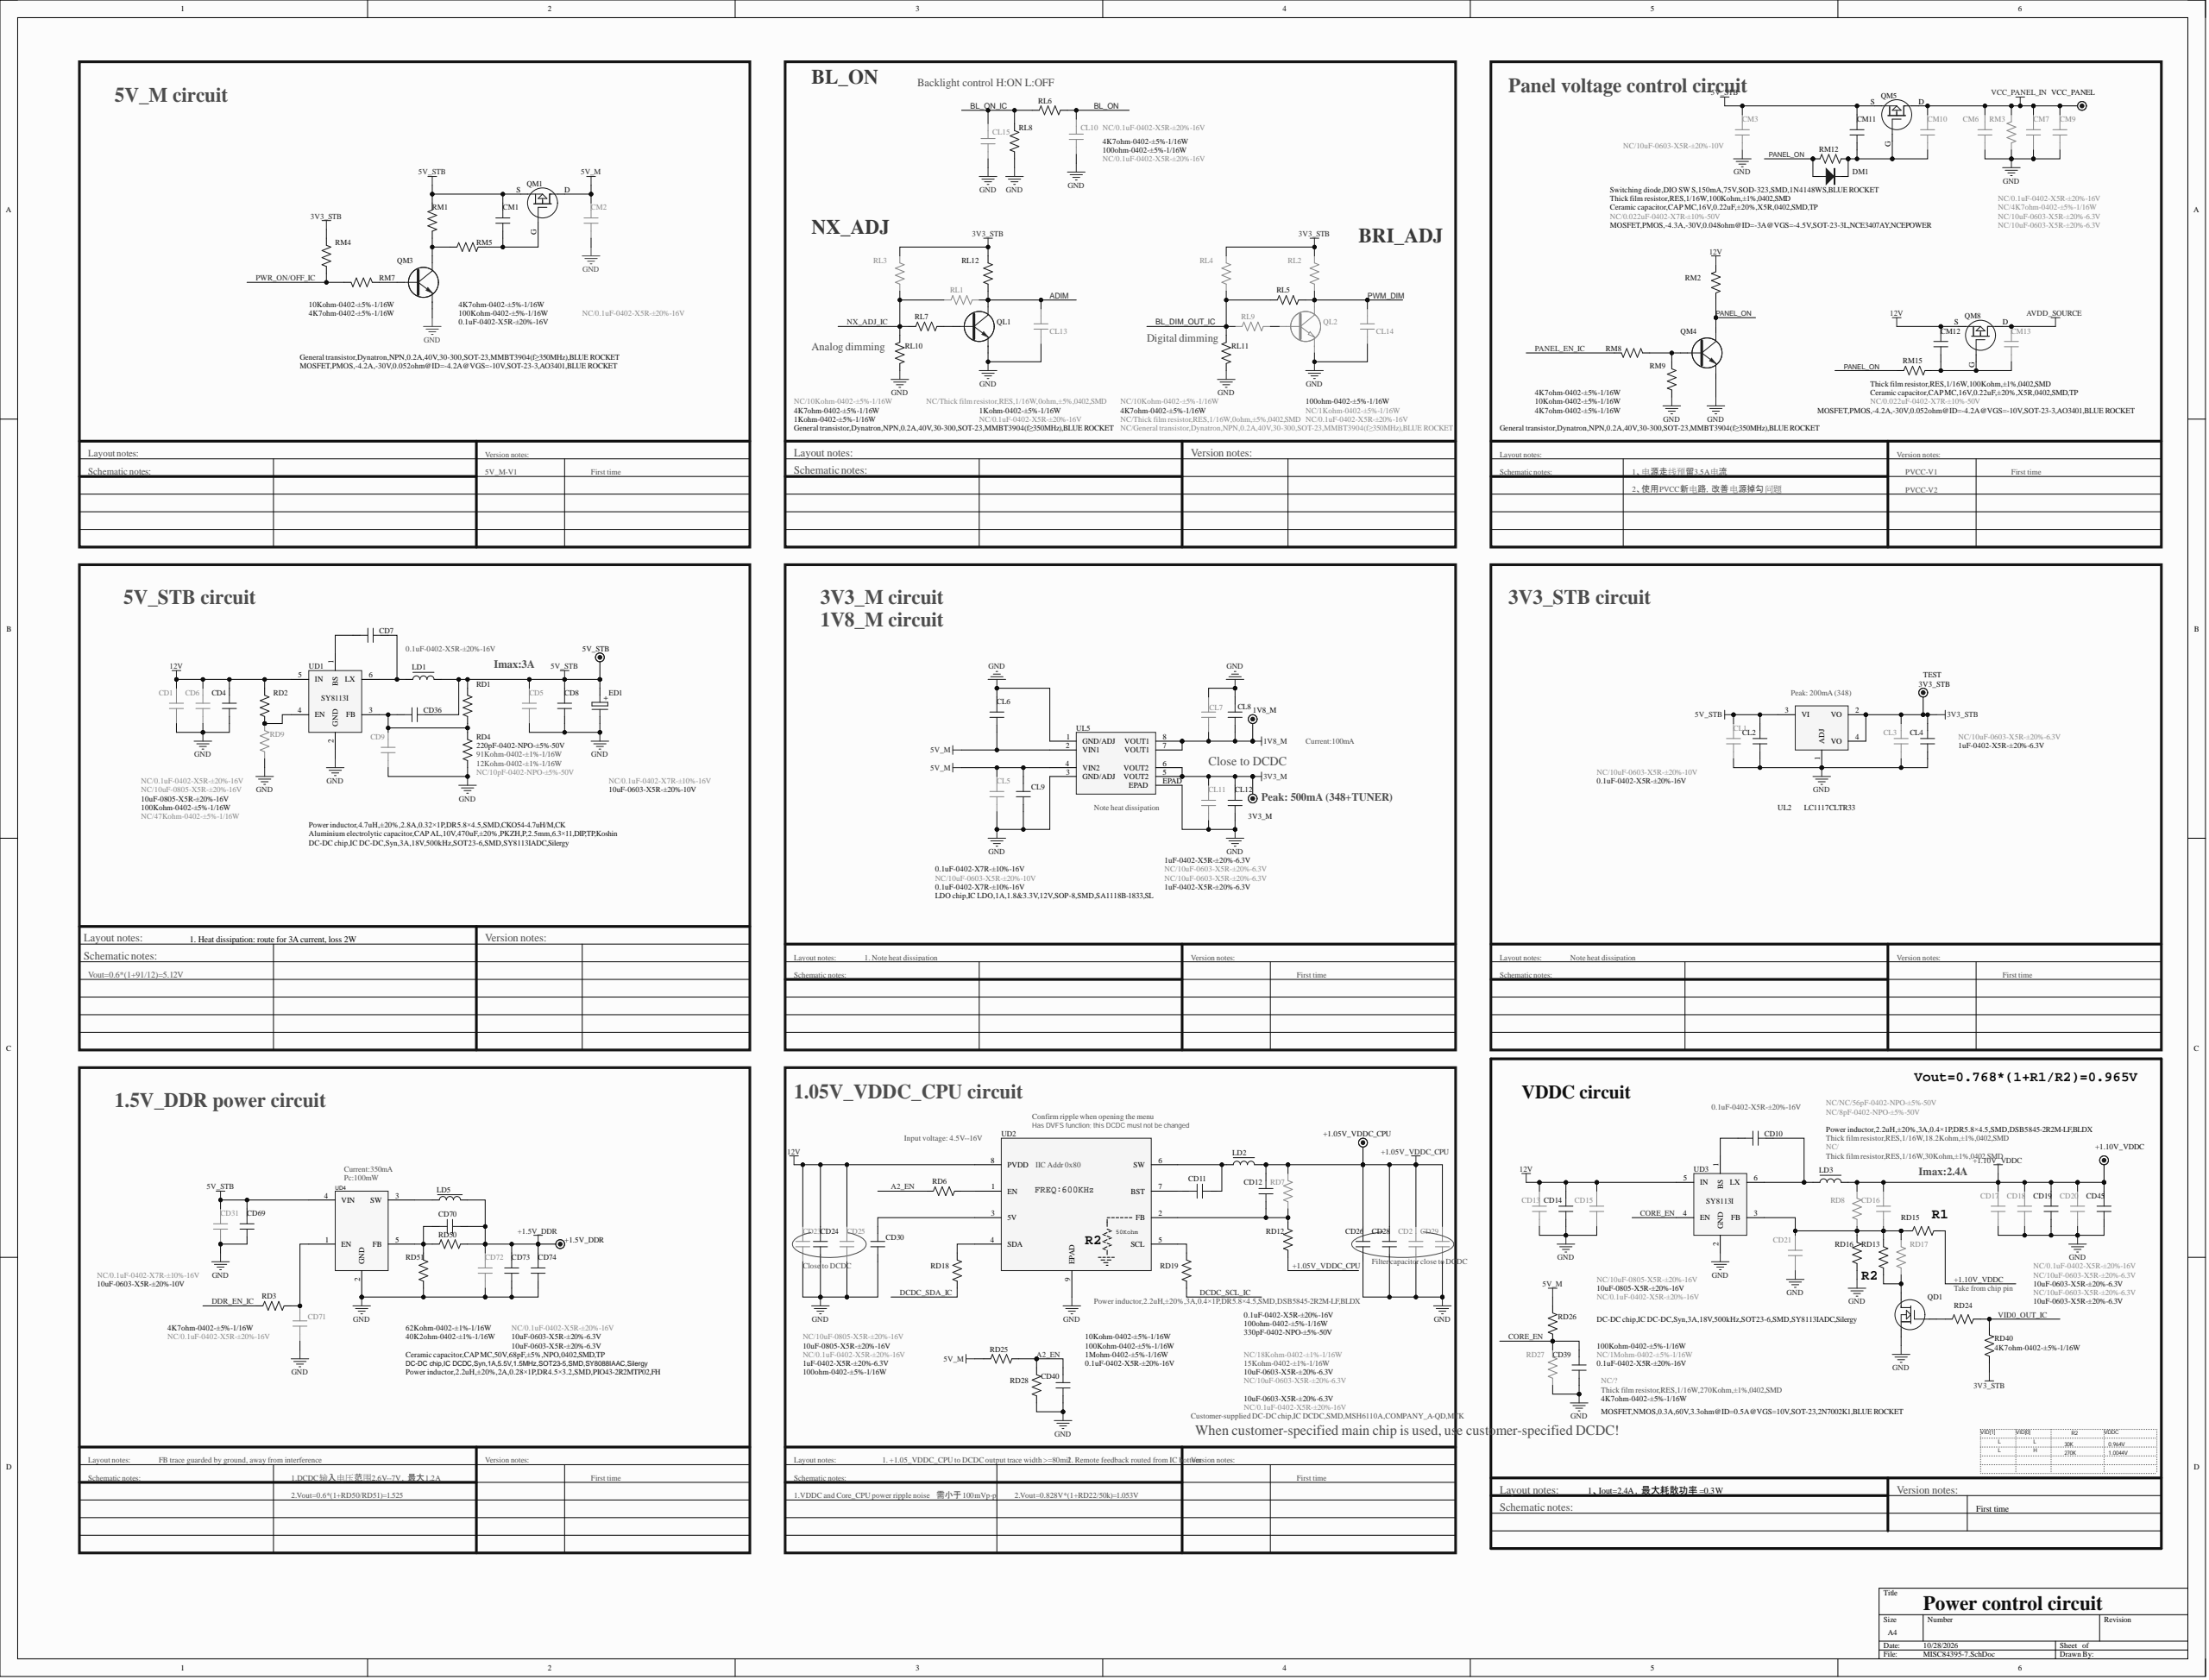Circuit board | Altium Designer | 951 parts | 509 nets | one sheet of the schematic
Parts on this sheet (reference | value | footprint):
1V8_M | TEST | TP
3V3_STB | TEST | TP
5V_STB | TEST | TP
+1.5V_DDR | TEST | TP
+1.05V_VDDC_CPU | TEST | TP
+1.10V_VDDC | TEST | TP
CD1 | NC/0.1uF-0402-X5R-±20%-16V | C0402
CD2 | NC/10uF-0603-X5R-±20%-6.3V | C0603
CD4 | 10uF-0805-X5R-±20%-16V | C0805
CD5 | NC/0.1uF-0402-X7R-±10%-16V | C0402
CD6 | NC/10uF-0805-X5R-±20%-16V | C0805
CD7 | 0.1uF-0402-X5R-±20%-16V | C0402
CD8 | 10uF-0603-X5R-±20%-10V | C0603
CD9 | NC/10pF-0402-NPO-±5%-50V | C0402
CD10 | 0.1uF-0402-X5R-±20%-16V | C0402
CD11 | 0.1uF-0402-X5R-±20%-16V | C0402
CD12 | 330pF-0402-NPO-±5%-50V | C0402
CD13 | NC/10uF-0805-X5R-±20%-16V | C0805
CD14 | 10uF-0805-X5R-±20%-16V | C0805
CD15 | NC/0.1uF-0402-X5R-±20%-16V | C0402
CD16 | NC/NC/56pF-0402-NPO-±5%-50V | C0402
CD17 | NC/0.1uF-0402-X5R-±20%-16V | C0402
CD18 | NC/10uF-0603-X5R-±20%-6.3V | C0603
CD19 | 10uF-0603-X5R-±20%-6.3V | C0603
CD20 | NC/10uF-0603-X5R-±20%-6.3V | C0603
CD21 | NC/8pF-0402-NPO-±5%-50V | C0402
CD23 | NC/10uF-0805-X5R-±20%-16V | C0805
CD24 | 10uF-0805-X5R-±20%-16V | C0805
CD25 | NC/0.1uF-0402-X5R-±20%-16V | C0402
CD26 | 10uF-0603-X5R-±20%-6.3V | C0603
CD28 | 10uF-0603-X5R-±20%-6.3V | C0603
CD29 | NC/0.1uF-0402-X5R-±20%-16V | C0402
CD30 | 1uF-0402-X5R-±20%-6.3V | C0402
CD31 | NC/0.1uF-0402-X7R-±10%-16V | C0402
CD36 | 220pF-0402-NPO-±5%-50V | C0402
CD39 | 0.1uF-0402-X5R-±20%-16V | C0402
CD40 | 0.1uF-0402-X5R-±20%-16V | C0402
CD45 | 10uF-0603-X5R-±20%-6.3V | C0603
CD69 | 10uF-0603-X5R-±20%-10V | C0603
CD70 | Ceramic capacitor,CAP MC,50V,68pF,±5%,NPO,0402,SMD,TP | C0402
CD71 | NC/0.1uF-0402-X5R-±20%-16V | C0402
CD72 | NC/0.1uF-0402-X5R-±20%-16V | C0402
CD73 | 10uF-0603-X5R-±20%-6.3V | C0603
CD74 | 10uF-0603-X5R-±20%-6.3V | C0603
CL1 | NC/10uF-0603-X5R-±20%-10V | C0603
CL2 | 0.1uF-0402-X5R-±20%-16V | C0402
CL3 | NC/10uF-0603-X5R-±20%-6.3V | C0603
CL4 | 1uF-0402-X5R-±20%-6.3V | C0402
CL5 | NC/10uF-0603-X5R-±20%-10V | C0603
CL6 | 0.1uF-0402-X7R-±10%-16V | C0402
CL7 | NC/10uF-0603-X5R-±20%-6.3V | C0603
CL8 | 1uF-0402-X5R-±20%-6.3V | C0402
CL9 | 0.1uF-0402-X7R-±10%-16V | C0402
CL10 | NC/0.1uF-0402-X5R-±20%-16V | C0402
CL11 | NC/10uF-0603-X5R-±20%-6.3V | C0603
CL12 | 1uF-0402-X5R-±20%-6.3V | C0402
CL13 | NC/0.1uF-0402-X5R-±20%-16V | C0402
CL14 | NC/0.1uF-0402-X5R-±20%-16V | C0402
CL15 | NC/0.1uF-0402-X5R-±20%-16V | C0402
CM1 | 0.1uF-0402-X5R-±20%-16V | C0402
CM2 | NC/0.1uF-0402-X5R-±20%-16V | C0402
CM3 | NC/10uF-0603-X5R-±20%-10V | C0603
CM6 | NC/0.1uF-0402-X5R-±20%-16V | C0402
CM7 | NC/10uF-0603-X5R-±20%-6.3V | C0603
CM9 | NC/10uF-0603-X5R-±20%-6.3V | C0603
CM10 | NC/0.022uF-0402-X7R-±10%-50V | C0402
CM11 | Ceramic capacitor,CAP MC,16V,0.22uF,±20%,X5R,0402,SMD,TP | C0402
CM12 | Ceramic capacitor,CAP MC,16V,0.22uF,±20%,X5R,0402,SMD,TP | C0402
CM13 | NC/0.022uF-0402-X7R-±10%-50V | C0402
DM1 | Switching diode,DIO SW S,150mA,75V,SOD-323,SMD,1N4148WS,BLUE ROCKET | DIODE-S-12
ED1 | Aluminium electrolytic capacitor,CAP AL,10V,470uF,±20%,PKZH,P,2.5mm,6.3×11,DIP,TP,Koshin | EC(6.3*11)-V-2.5
LD1 | Power inductor,4.7uH,±20%,2.8A,0.32×1P,DR5.8×4.5,SMD,CKO54-4.7uH/M,CK | L(6.0*4.5)-S
LD2 | Power inductor,2.2uH,±20%,3A,0.4×1P,DR5.8×4.5,SMD,DSB5845-2R2M-LF,BLDX | L(5.8*4.5)-S
LD3 | Power inductor,2.2uH,±20%,3A,0.4×1P,DR5.8×4.5,SMD,DSB5845-2R2M-LF,BLDX | L(5.8*4.5)-S
LD5 | Power inductor,2.2uH,±20%,2A,0.28×1P,DR4.5×3.2,SMD,PIO43-2R2MTP02,FH | L(4.5*3.5)-S
QD1 | MOSFET,NMOS,0.3A,60V,3.3ohm@ID=0.5A@VGS=10V,SOT-23,2N7002K1,BLUE ROCKET | SOT-23-7
QL1 | General transistor,Dynatron,NPN,0.2A,40V,30-300,SOT-23,MMBT3904(f=350MHz),BLUE ROCKET | SOT-23
QL2 | NC/General transistor,Dynatron,NPN,0.2A,40V,30-300,SOT-23,MMBT3904(f=350MHz),BLUE ROCKET | SOT-23
QM1 | MOSFET,PMOS,-4.2A,-30V,0.052ohm@ID=-4.2A@VGS=-10V,SOT-23-3,AO3401,BLUE ROCKET | SOT-23-1
QM3 | General transistor,Dynatron,NPN,0.2A,40V,30-300,SOT-23,MMBT3904(f=350MHz),BLUE ROCKET | SOT-23
QM4 | General transistor,Dynatron,NPN,0.2A,40V,30-300,SOT-23,MMBT3904(f=350MHz),BLUE ROCKET | SOT-23
QM5 | MOSFET,PMOS,-4.3A,-30V,0.048ohm@ID=-3A@VGS=-4.5V,SOT-23-3L,NCE3407AY,NCEPOWER | SOT-23-1
QM8 | MOSFET,PMOS,-4.2A,-30V,0.052ohm@ID=-4.2A@VGS=-10V,SOT-23-3,AO3401,BLUE ROCKET | SOT-23-1
RD1 | 91Kohm-0402-±1%-1/16W | R0402
RD2 | 100Kohm-0402-±5%-1/16W | R0402
RD3 | 4K7ohm-0402-±5%-1/16W | R0402
RD4 | 12Kohm-0402-±1%-1/16W | R0402
RD6 | 10Kohm-0402-±5%-1/16W | R0402
RD7 | NC/18Kohm-0402-±1%-1/16W | R0402
RD8 | NC/ | R0402
RD9 | NC/47Kohm-0402-±5%-1/16W | R0402
RD12 | 15Kohm-0402-±1%-1/16W | R0402
RD13 | Thick film resistor,RES,1/16W,270Kohm,±1%,0402,SMD | R0402
RD15 | Thick film resistor,RES,1/16W,18.2Kohm,±1%,0402,SMD | R0402
RD16 | Thick film resistor,RES,1/16W,30Kohm,±1%,0402,SMD | R0402
RD17 | NC/? | R0402
RD18 | 100ohm-0402-±5%-1/16W | R0402
RD19 | 100ohm-0402-±5%-1/16W | R0402
RD24 | 4K7ohm-0402-±5%-1/16W | R0402
RD25 | 100Kohm-0402-±5%-1/16W | R0402
RD26 | 100Kohm-0402-±5%-1/16W | R0402
RD27 | NC/1Mohm-0402-±5%-1/16W | R0402
RD28 | 1Mohm-0402-±5%-1/16W | R0402
RD40 | 4K7ohm-0402-±5%-1/16W | R0402
RD50 | 62Kohm-0402-±1%-1/16W | R0402
RD51 | 40K2ohm-0402-±1%-1/16W | R0402
RL1 | NC/Thick film resistor,RES,1/16W,0ohm,±5%,0402,SMD | R0402
RL2 | NC/1Kohm-0402-±5%-1/16W | R0402
RL3 | NC/10Kohm-0402-±5%-1/16W | R0402
RL4 | NC/10Kohm-0402-±5%-1/16W | R0402
RL5 | 100ohm-0402-±5%-1/16W | R0402
RL6 | 100ohm-0402-±5%-1/16W | R0402
RL7 | 1Kohm-0402-±5%-1/16W | R0402
RL8 | 4K7ohm-0402-±5%-1/16W | R0402
RL9 | NC/Thick film resistor,RES,1/16W,0ohm,±5%,0402,SMD | R0402
RL10 | 4K7ohm-0402-±5%-1/16W | R0402
RL11 | 4K7ohm-0402-±5%-1/16W | R0402
RL12 | 1Kohm-0402-±5%-1/16W | R0402
RM1 | 4K7ohm-0402-±5%-1/16W | R0402
RM2 | 4K7ohm-0402-±5%-1/16W | R0402
RM3 | NC/4K7ohm-0402-±5%-1/16W | R0402
RM4 | 10Kohm-0402-±5%-1/16W | R0402
RM5 | 100Kohm-0402-±5%-1/16W | R0402
RM7 | 4K7ohm-0402-±5%-1/16W | R0402
RM8 | 4K7ohm-0402-±5%-1/16W | R0402
RM9 | 10Kohm-0402-±5%-1/16W | R0402
RM12 | Thick film resistor,RES,1/16W,100Kohm,±1%,0402,SMD | R0402
RM15 | Thick film resistor,RES,1/16W,100Kohm,±1%,0402,SMD | R0402
UD1 | DC-DC chip,IC DC-DC,Syn,3A,18V,500kHz,SOT23-6,SMD,SY8113IADC,Silergy | TSOT23-6
UD2 | Customer-supplied DC-DC chip,IC DCDC,SMD,MSH6110A,COMPANY_A-QD,MTK | SOP8/1.27
UD3 | DC-DC chip,IC DC-DC,Syn,3A,18V,500kHz,SOT23-6,SMD,SY8113IADC,Silergy | TSOT23-6
UD4 | DC-DC chip,IC DCDC,Syn,1A,5.5V,1.5MHz,SOT23-5,SMD,SY8088IAAC,Silergy | SOT-23-5
UL2 | LC1117CLTR33 | SOT-223
UL5 | LDO chip,IC LDO,1A,1.8&3.3V,12V,SOP-8,SMD,SA1118B-1833,SL | SOP8/1.27-3
VCC_PANEL | TEST | TP
Nets of these parts (net: part-pin ...):
VID0_OUT_IC: RD24-2 RD40-1
VCC_PANEL_IN: CM6-2 CM7-2 CM9-2 CM10-1 QM5-D RM3-1 VCC_PANEL-1
PWR_ON/OFF_IC: RM4-2 RM7-1
PWM_DIM: CL14-2 QL2-C RL2-1 RL5-1
PANEL_ON: DM1-A QM4-C RM2-2 RM12-1 RM15-1
PANEL_EN_IC: RM8-1
NX_ADJ_IC: RL1-1 RL3-1 RL7-2 RL10-1
NetRD19_1: RD19-1 UD2-5
NetRD18_1: RD18-1 UD2-4
NetRD6_2: RD6-2 UD2-1
NetRD2_2: RD2-2 RD9-2 UD1-4
NetQM4_B: QM4-B RM8-2 RM9-1
NetQM3_C: QM3-C RM1-1 RM5-1
NetQM3_B: QM3-B RM7-2
NetQL2_B: QL2-B RL9-1
NetQL1_B: QL1-B RL7-1
NetQD1_G: QD1-G RD24-1
NetQD1_D: QD1-D RD13-1 RD17-1
NetLD5_1: LD5-1 UD4-3
NetCM12_1: CM12-1 CM13-2 QM8-G RM15-2
NetCM10_2: CM10-2 CM11-1 DM1-K QM5-G RM12-2
NetCM1_2: CM1-2 QM1-G RM5-2
NetCD71_2: CD71-2 RD3-1 UD4-1
NetCD70_1: CD70-1 RD50-1 RD51-2 UD4-5
NetCD30_1: CD30-1 UD2-3
NetCD16_1: CD16-1 CD21-1 RD8-1 RD13-2 RD15-2 RD16-2 RD17-2 UD3-3
NetCD12_1: CD12-1 RD7-1 RD12-1 UD2-2
NetCD11_2: CD11-2 UD2-7
NetCD11_1: CD11-1 LD2-1 UD2-6
NetCD10_2: CD10-2 LD3-1 UD3-6
NetCD10_1: CD10-1 UD3-1
NetCD9_1: CD9-1 CD36-1 RD1-1 RD4-2 UD1-3
NetCD7_2: CD7-2 LD1-1 UD1-6
NetCD7_1: CD7-1 UD1-1
GND: CD1-1 CD2-1 CD4-2 CD5-2 CD6-2 CD8-1 CD9-2 CD13-2 CD14-2 CD15-2 CD17-2 CD18-2 CD19-2 CD20-2 CD21-2 CD23-1 CD24-1 CD25-1 CD26-1 CD28-1 CD29-2 CD30-2 CD31-1 CD39-2 CD40-2 CD45-2 CD69-1 CD71-1 CD72-1 CD73-2 CD74-2 CL1-1 CL2-2 CL3-2 CL4-2 CL5-1 CL6-1 CL7-1 CL8-1 CL9-1 CL10-1 CL11-2 CL12-2 CL13-1 CL14-1 CL15-1 CM2-2 CM3-1 CM6-1 CM7-1 CM9-1 ED1-2 QD1-S QL1-E QL2-E QM3-E QM4-E RD4-1 RD9-1 RD16-1 RD27-2 RD28-2 RD51-1 RL8-1 RL10-2 RL11-2 RM3-2 RM9-2 UD1-2 UD2-9 UD3-2 UD4-2 UL2-1 UL5-1 UL5-3 UL5-EPAD
DDR_EN_IC: RD3-2
DCDC_SDA_IC: RD18-2
DCDC_SCL_IC: RD19-2
CORE_EN: CD39-1 RD26-1 RD27-1 UD3-4
BL_ON_IC: CL15-2 RL6-2 RL8-2
BL_ON: CL10-2 RL6-1
BL_DIM_OUT_IC: RL4-1 RL5-2 RL9-2 RL11-1
AVDD_SOURCE: CM13-1 QM8-D
ADIM: CL13-2 QL1-C RL1-2 RL12-1
A2_EN: CD40-1 RD6-1 RD25-1 RD28-1
+1.10V_VDDC: +1.10V_VDDC-1 CD16-2 CD17-1 CD18-1 CD19-1 CD20-1 CD45-1 LD3-2 RD8-2 RD15-1
+1.05V_VDDC_CPU: +1.05V_VDDC_CPU-1 CD2-2 CD12-2 CD26-2 CD28-2 CD29-1 LD2-2 RD7-2 RD12-2
+1.5V_DDR: +1.5V_DDR-1 CD70-2 CD72-2 CD73-1 CD74-1 LD5-2 RD50-2
12V: CD1-2 CD4-1 CD6-1 CD13-1 CD14-1 CD15-1 CD23-2 CD24-2 CD25-2 CM12-2 QM8-S RD2-1 RM2-1 UD1-5 UD2-8 UD3-5
5V_STB: 5V_STB-1 CD5-1 CD8-2 CD31-2 CD36-2 CD69-2 CL1-2 CL2-1 CM1-1 CM3-2 CM11-2 ED1-1 LD1-2 QM1-S QM5-S RD1-2 RM1-2 UD4-4 UL2-3
5V_M: CL5-2 CL6-2 CL9-2 CM2-1 QM1-D RD25-2 RD26-2 UL5-2 UL5-4
3V3_STB: 3V3_STB-1 CL3-1 CL4-1 RD40-2 RL2-2 RL3-2 RL4-2 RL12-2 RM4-1 UL2-2 UL2-4
3V3_M: CL11-1 CL12-1 UL5-5 UL5-6
1V8_M: 1V8_M-1 CL7-2 CL8-2 UL5-7 UL5-8